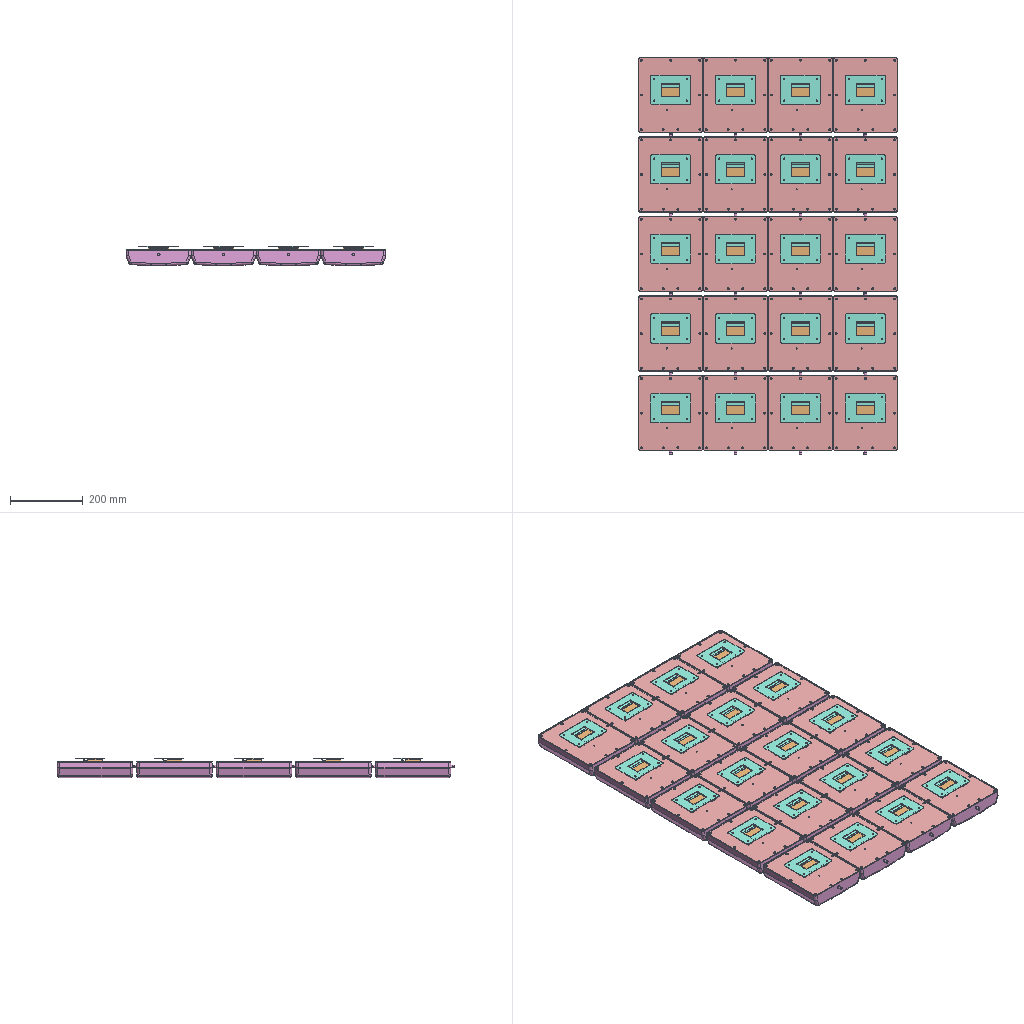Assembly | SolidWorks | 6 different items | 120 placed | box 712 x 1090 x 54 mm
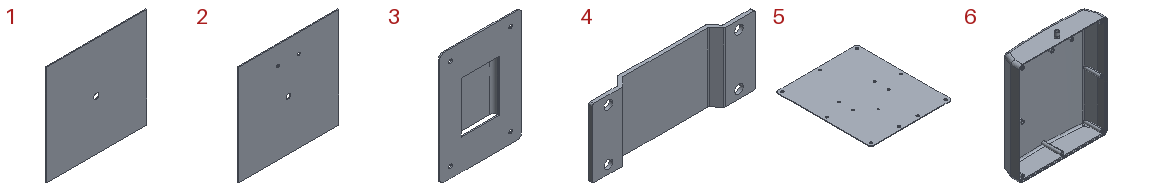Parts list (item | quantity | size | volume | features):
1 | x20 | 98.4 x 0.8 x 98.4 mm | 7730 mm3 | features Extrusion 1
2 | x20 | 110.5 x 1 x 110.5 mm | 12176 mm3 | features Extrusion 1
3 | x20 | 80 x 6.2 x 110 mm | 10376 mm3 | features FlatPattern 1, ICE 1, SMBaseFlange 1, SheetMetal 1
4 | x20 | 95 x 7 x 40 mm | 7797 mm3 | features Extrusion 1, Fillet 1, ICE 1
5 | x20 | 175 x 204 x 31.2 mm | 42842 mm3 | features Chamfer 2, Extrusion 1, Helix 1, ICE 1, SweepCut 1
6 | x20 | 178 x 44 x 217.6 mm | 217327 mm3 | features ICE 2, Extrusion 1, Fillet 1, Revolution 1, Shell 1
Mates (type | each side: item.copy, entity, surface, feature):
Concentric | 5.1 face cylinder Boss-Extrude2 | 2.1 face cylinder Boss-Extrude1
Parallel | 5.1 face plane Boss-Extrude1 | 2.1 face plane Boss-Extrude1
Concentric | 5.1 face cylinder Boss-Extrude2 | 1.1 face cylinder Boss-Extrude1
Parallel | 2.1 face plane Boss-Extrude1 | 1.1 face plane Boss-Extrude1
Concentric | 5.1 face cylinder Boss-Extrude1 | 6.1 face cylinder Boss-Extrude3 | 2 times
Coincident | 5.1 face plane Boss-Extrude1 | 6.1 face plane Boss-Extrude1
Parallel | 5.1 face plane Boss-Extrude1 | 4.1 face plane Boss-Extrude1
Concentric | 5.1 face cylinder Boss-Extrude1 | 4.1 face cylinder Cut-Extrude1
Coincident | 5.1 face plane Boss-Extrude1 | 4.1 face plane Boss-Extrude1
Parallel | 6.1 face plane Boss-Extrude1 | 4.1 face plane Boss-Extrude1
DistanceDim | 3.1 face plane Boss-Extrude1 | 4.1 face plane Boss-Extrude1
Coincident | 3.1 face plane Boss-Extrude1 | 4.1 face plane Boss-Extrude1
Width | 6.1 face plane Boss-Extrude1 | 6.1 face plane Boss-Extrude1 | 3.1 face plane Base-Flange1 | 3.1 face plane Base-Flange1